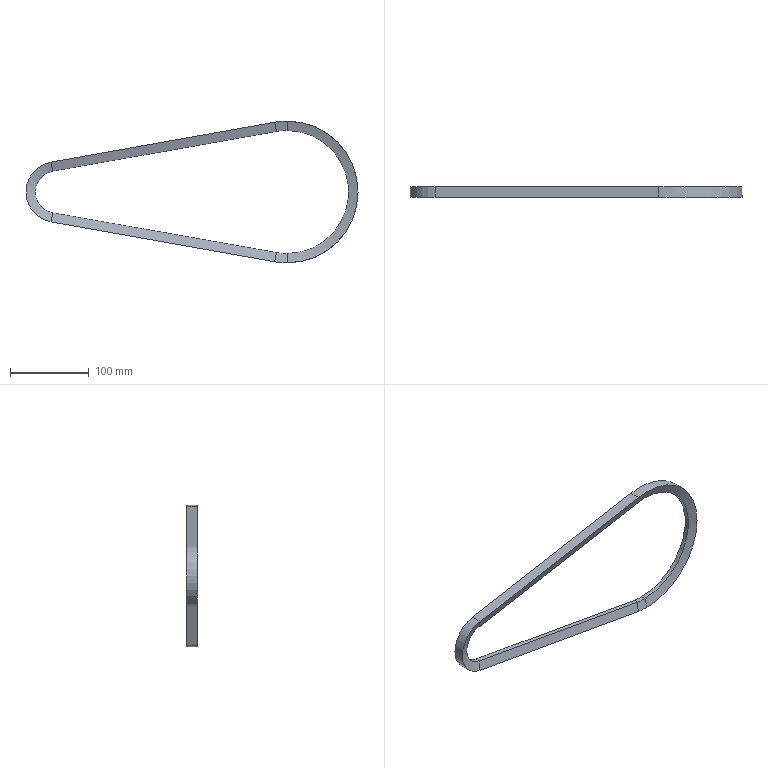Part | SolidWorks | features BaseBody 1 | 1 solid | 22 faces | box 421.873 x 13.3 x 180 mm | volume 107994 mm3 | plane 8 | cone 7 | cylinder 7 | commonest cylinder face diameters 156.432 x3 180 x2 53.781 x1 77.349 x1
STEP:
#1=CARTESIAN_POINT('',(-26.891,2.821,0.));
#2=VERTEX_POINT('',#1);
#3=CARTESIAN_POINT('',(-4.707,2.821,26.475));
#4=VERTEX_POINT('',#3);
#5=CARTESIAN_POINT('',(0.,2.821,0.));
#6=DIRECTION('',(0.,1.,0.));
#7=DIRECTION('',(0.1751,0.,-0.9846));
#8=AXIS2_PLACEMENT_3D('',#5,#6,#7);
#9=CIRCLE('',#8,26.891);
#10=EDGE_CURVE('',#2,#4,#9,.T.);
#11=ORIENTED_EDGE('',*,*,#10,.F.);
#12=CARTESIAN_POINT('',(-38.675,6.65,0.));
#13=VERTEX_POINT('',#12);
#14=CARTESIAN_POINT('',(-38.675,6.65,0.));
#15=DIRECTION('',(-0.9511,0.309,0.));
#16=VECTOR('',#15,1000.);
#17=LINE('',#14,#16);
#18=EDGE_CURVE('',#2,#13,#17,.T.);
#19=ORIENTED_EDGE('',*,*,#18,.T.);
#20=CARTESIAN_POINT('',(-6.77,6.65,38.078));
#21=VERTEX_POINT('',#20);
#22=CARTESIAN_POINT('',(0.,6.65,0.));
#23=DIRECTION('',(0.,-1.,0.));
#24=DIRECTION('',(0.1751,0.,-0.9846));
#25=AXIS2_PLACEMENT_3D('',#22,#23,#24);
#26=CIRCLE('',#25,38.675);
#27=EDGE_CURVE('',#21,#13,#26,.T.);
#28=ORIENTED_EDGE('',*,*,#27,.F.);
#29=CARTESIAN_POINT('',(-5.739,4.736,32.276));
#30=DIRECTION('',(-0.1665,0.309,0.9364));
#31=VECTOR('',#30,1000.);
#32=LINE('',#29,#31);
#33=EDGE_CURVE('',#4,#21,#32,.T.);
#34=ORIENTED_EDGE('',*,*,#33,.F.);
#35=EDGE_LOOP('',(#11,#19,#28,#34));
#36=FACE_OUTER_BOUND('',#35,.T.);
#37=CARTESIAN_POINT('',(0.,6.65,0.));
#38=DIRECTION('',(0.,1.,0.));
#39=DIRECTION('',(-1.,0.,0.));
#40=AXIS2_PLACEMENT_3D('',#37,#38,#39);
#41=CONICAL_SURFACE('',#40,38.675,1.257);
#42=ADVANCED_FACE('',(#36),#41,.F.);
#43=CARTESIAN_POINT('',(279.506,2.821,77.008));
#44=VERTEX_POINT('',#43);
#45=CARTESIAN_POINT('',(293.198,2.821,78.216));
#46=VERTEX_POINT('',#45);
#47=CARTESIAN_POINT('',(293.198,2.821,0.));
#48=DIRECTION('',(0.,1.,0.));
#49=DIRECTION('',(0.1751,0.,0.9846));
#50=AXIS2_PLACEMENT_3D('',#47,#48,#49);
#51=CIRCLE('',#50,78.216);
#52=EDGE_CURVE('',#44,#46,#51,.T.);
#53=ORIENTED_EDGE('',*,*,#52,.T.);
#54=CARTESIAN_POINT('',(293.198,-2.821,78.216));
#55=VERTEX_POINT('',#54);
#56=CARTESIAN_POINT('',(293.198,2.821,78.216));
#57=DIRECTION('',(0.,-1.,0.));
#58=VECTOR('',#57,1000.);
#59=LINE('',#56,#58);
#60=EDGE_CURVE('',#46,#55,#59,.T.);
#61=ORIENTED_EDGE('',*,*,#60,.T.);
#62=CARTESIAN_POINT('',(279.506,-2.821,77.008));
#63=VERTEX_POINT('',#62);
#64=CARTESIAN_POINT('',(293.198,-2.821,0.));
#65=DIRECTION('',(0.,1.,0.));
#66=DIRECTION('',(0.1751,0.,0.9846));
#67=AXIS2_PLACEMENT_3D('',#64,#65,#66);
#68=CIRCLE('',#67,78.216);
#69=EDGE_CURVE('',#63,#55,#68,.T.);
#70=ORIENTED_EDGE('',*,*,#69,.F.);
#71=CARTESIAN_POINT('',(279.506,0.,77.008));
#72=DIRECTION('',(0.,-1.,0.));
#73=VECTOR('',#72,1000.);
#74=LINE('',#71,#73);
#75=EDGE_CURVE('',#44,#63,#74,.T.);
#76=ORIENTED_EDGE('',*,*,#75,.F.);
#77=EDGE_LOOP('',(#53,#61,#70,#76));
#78=FACE_OUTER_BOUND('',#77,.T.);
#79=CARTESIAN_POINT('',(293.198,2.821,0.));
#80=DIRECTION('',(0.,-1.,0.));
#81=DIRECTION('',(0.,0.,-1.));
#82=AXIS2_PLACEMENT_3D('',#79,#80,#81);
#83=CYLINDRICAL_SURFACE('',#82,78.216);
#84=ADVANCED_FACE('',(#78),#83,.F.);
#85=ORIENTED_EDGE('',*,*,#60,.F.);
#86=CARTESIAN_POINT('',(293.198,2.821,-78.216));
#87=VERTEX_POINT('',#86);
#88=CARTESIAN_POINT('',(293.198,2.821,0.));
#89=DIRECTION('',(0.,1.,0.));
#90=DIRECTION('',(0.1751,0.,0.9846));
#91=AXIS2_PLACEMENT_3D('',#88,#89,#90);
#92=CIRCLE('',#91,78.216);
#93=EDGE_CURVE('',#46,#87,#92,.T.);
#94=ORIENTED_EDGE('',*,*,#93,.T.);
#95=CARTESIAN_POINT('',(293.198,-2.821,-78.216));
#96=VERTEX_POINT('',#95);
#97=CARTESIAN_POINT('',(293.198,2.821,-78.216));
#98=DIRECTION('',(0.,-1.,0.));
#99=VECTOR('',#98,1000.);
#100=LINE('',#97,#99);
#101=EDGE_CURVE('',#87,#96,#100,.T.);
#102=ORIENTED_EDGE('',*,*,#101,.T.);
#103=CARTESIAN_POINT('',(293.198,-2.821,0.));
#104=DIRECTION('',(0.,1.,0.));
#105=DIRECTION('',(0.1751,0.,0.9846));
#106=AXIS2_PLACEMENT_3D('',#103,#104,#105);
#107=CIRCLE('',#106,78.216);
#108=EDGE_CURVE('',#55,#96,#107,.T.);
#109=ORIENTED_EDGE('',*,*,#108,.F.);
#110=EDGE_LOOP('',(#85,#94,#102,#109));
#111=FACE_OUTER_BOUND('',#110,.T.);
#112=CARTESIAN_POINT('',(293.198,2.821,0.));
#113=DIRECTION('',(0.,-1.,0.));
#114=DIRECTION('',(0.,0.,-1.));
#115=AXIS2_PLACEMENT_3D('',#112,#113,#114);
#116=CYLINDRICAL_SURFACE('',#115,78.216);
#117=ADVANCED_FACE('',(#111),#116,.F.);
#118=CARTESIAN_POINT('',(277.443,6.65,-88.61));
#119=VERTEX_POINT('',#118);
#120=CARTESIAN_POINT('',(383.198,6.65,0.));
#121=VERTEX_POINT('',#120);
#122=CARTESIAN_POINT('',(293.198,6.65,0.));
#123=DIRECTION('',(0.,-1.,0.));
#124=DIRECTION('',(0.1751,0.,0.9846));
#125=AXIS2_PLACEMENT_3D('',#122,#123,#124);
#126=CIRCLE('',#125,90.);
#127=EDGE_CURVE('',#119,#121,#126,.T.);
#128=ORIENTED_EDGE('',*,*,#127,.T.);
#129=CARTESIAN_POINT('',(383.198,-6.65,0.));
#130=VERTEX_POINT('',#129);
#131=CARTESIAN_POINT('',(383.198,6.65,0.));
#132=DIRECTION('',(0.,-1.,0.));
#133=VECTOR('',#132,1000.);
#134=LINE('',#131,#133);
#135=EDGE_CURVE('',#121,#130,#134,.T.);
#136=ORIENTED_EDGE('',*,*,#135,.T.);
#137=CARTESIAN_POINT('',(293.198,-6.65,-90.));
#138=VERTEX_POINT('',#137);
#139=CARTESIAN_POINT('',(293.198,-6.65,0.));
#140=DIRECTION('',(0.,-1.,0.));
#141=DIRECTION('',(0.1751,0.,0.9846));
#142=AXIS2_PLACEMENT_3D('',#139,#140,#141);
#143=CIRCLE('',#142,90.);
#144=EDGE_CURVE('',#138,#130,#143,.T.);
#145=ORIENTED_EDGE('',*,*,#144,.F.);
#146=CARTESIAN_POINT('',(277.443,-6.65,-88.61));
#147=VERTEX_POINT('',#146);
#148=CARTESIAN_POINT('',(293.198,-6.65,0.));
#149=DIRECTION('',(0.,-1.,0.));
#150=DIRECTION('',(0.1751,0.,0.9846));
#151=AXIS2_PLACEMENT_3D('',#148,#149,#150);
#152=CIRCLE('',#151,90.);
#153=EDGE_CURVE('',#147,#138,#152,.T.);
#154=ORIENTED_EDGE('',*,*,#153,.F.);
#155=CARTESIAN_POINT('',(277.443,0.,-88.61));
#156=DIRECTION('',(0.,1.,0.));
#157=VECTOR('',#156,1000.);
#158=LINE('',#155,#157);
#159=EDGE_CURVE('',#147,#119,#158,.T.);
#160=ORIENTED_EDGE('',*,*,#159,.T.);
#161=EDGE_LOOP('',(#128,#136,#145,#154,#160));
#162=FACE_OUTER_BOUND('',#161,.T.);
#163=CARTESIAN_POINT('',(293.198,6.65,0.));
#164=DIRECTION('',(0.,-1.,0.));
#165=DIRECTION('',(1.,0.,0.));
#166=AXIS2_PLACEMENT_3D('',#163,#164,#165);
#167=CYLINDRICAL_SURFACE('',#166,90.);
#168=ADVANCED_FACE('',(#162),#167,.T.);
#169=ORIENTED_EDGE('',*,*,#69,.T.);
#170=CARTESIAN_POINT('',(293.198,-6.65,90.));
#171=VERTEX_POINT('',#170);
#172=CARTESIAN_POINT('',(293.198,-2.821,78.216));
#173=DIRECTION('',(0.,-0.309,0.9511));
#174=VECTOR('',#173,1000.);
#175=LINE('',#172,#174);
#176=EDGE_CURVE('',#55,#171,#175,.T.);
#177=ORIENTED_EDGE('',*,*,#176,.T.);
#178=CARTESIAN_POINT('',(277.443,-6.65,88.61));
#179=VERTEX_POINT('',#178);
#180=CARTESIAN_POINT('',(293.198,-6.65,0.));
#181=DIRECTION('',(0.,-1.,0.));
#182=DIRECTION('',(0.1751,0.,0.9846));
#183=AXIS2_PLACEMENT_3D('',#180,#181,#182);
#184=CIRCLE('',#183,90.);
#185=EDGE_CURVE('',#171,#179,#184,.T.);
#186=ORIENTED_EDGE('',*,*,#185,.T.);
#187=CARTESIAN_POINT('',(278.475,-4.736,82.809));
#188=DIRECTION('',(-0.1665,-0.309,0.9364));
#189=VECTOR('',#188,1000.);
#190=LINE('',#187,#189);
#191=EDGE_CURVE('',#63,#179,#190,.T.);
#192=ORIENTED_EDGE('',*,*,#191,.F.);
#193=EDGE_LOOP('',(#169,#177,#186,#192));
#194=FACE_OUTER_BOUND('',#193,.T.);
#195=CARTESIAN_POINT('',(293.198,-2.821,0.));
#196=DIRECTION('',(0.,-1.,0.));
#197=DIRECTION('',(0.,0.,-1.));
#198=AXIS2_PLACEMENT_3D('',#195,#196,#197);
#199=CONICAL_SURFACE('',#198,78.216,1.257);
#200=ADVANCED_FACE('',(#194),#199,.F.);
#201=ORIENTED_EDGE('',*,*,#176,.F.);
#202=ORIENTED_EDGE('',*,*,#108,.T.);
#203=CARTESIAN_POINT('',(293.198,-2.821,-78.216));
#204=DIRECTION('',(0.,-0.309,-0.9511));
#205=VECTOR('',#204,1000.);
#206=LINE('',#203,#205);
#207=EDGE_CURVE('',#96,#138,#206,.T.);
#208=ORIENTED_EDGE('',*,*,#207,.T.);
#209=ORIENTED_EDGE('',*,*,#144,.T.);
#210=CARTESIAN_POINT('',(293.198,-6.65,0.));
#211=DIRECTION('',(0.,-1.,0.));
#212=DIRECTION('',(0.1751,0.,0.9846));
#213=AXIS2_PLACEMENT_3D('',#210,#211,#212);
#214=CIRCLE('',#213,90.);
#215=EDGE_CURVE('',#130,#171,#214,.T.);
#216=ORIENTED_EDGE('',*,*,#215,.T.);
#217=EDGE_LOOP('',(#201,#202,#208,#209,#216));
#218=FACE_OUTER_BOUND('',#217,.T.);
#219=CARTESIAN_POINT('',(293.198,-2.821,0.));
#220=DIRECTION('',(0.,-1.,0.));
#221=DIRECTION('',(0.,0.,-1.));
#222=AXIS2_PLACEMENT_3D('',#219,#220,#221);
#223=CONICAL_SURFACE('',#222,78.216,1.257);
#224=ADVANCED_FACE('',(#218),#223,.F.);
#225=CARTESIAN_POINT('',(279.506,2.821,-77.008));
#226=VERTEX_POINT('',#225);
#227=CARTESIAN_POINT('',(278.475,4.736,-82.809));
#228=DIRECTION('',(0.1665,-0.309,0.9364));
#229=VECTOR('',#228,1000.);
#230=LINE('',#227,#229);
#231=EDGE_CURVE('',#119,#226,#230,.T.);
#232=ORIENTED_EDGE('',*,*,#231,.F.);
#233=CARTESIAN_POINT('',(-6.77,6.65,-38.078));
#234=VERTEX_POINT('',#233);
#235=CARTESIAN_POINT('',(135.337,6.65,-63.344));
#236=DIRECTION('',(0.9846,0.,-0.1751));
#237=VECTOR('',#236,1000.);
#238=LINE('',#235,#237);
#239=EDGE_CURVE('',#234,#119,#238,.T.);
#240=ORIENTED_EDGE('',*,*,#239,.F.);
#241=CARTESIAN_POINT('',(-4.707,2.821,-26.475));
#242=VERTEX_POINT('',#241);
#243=CARTESIAN_POINT('',(-5.739,4.736,-32.276));
#244=DIRECTION('',(-0.1665,0.309,-0.9364));
#245=VECTOR('',#244,1000.);
#246=LINE('',#243,#245);
#247=EDGE_CURVE('',#242,#234,#246,.T.);
#248=ORIENTED_EDGE('',*,*,#247,.F.);
#249=CARTESIAN_POINT('',(137.399,2.821,-51.742));
#250=DIRECTION('',(-0.9846,0.,0.1751));
#251=VECTOR('',#250,1000.);
#252=LINE('',#249,#251);
#253=EDGE_CURVE('',#226,#242,#252,.T.);
#254=ORIENTED_EDGE('',*,*,#253,.F.);
#255=EDGE_LOOP('',(#232,#240,#248,#254));
#256=FACE_OUTER_BOUND('',#255,.T.);
#257=CARTESIAN_POINT('',(-12.554,6.835,-37.626));
#258=DIRECTION('',(0.05409,0.9511,0.3042));
#259=DIRECTION('',(0.1665,-0.309,0.9364));
#260=AXIS2_PLACEMENT_3D('',#257,#258,#259);
#261=PLANE('',#260);
#262=ADVANCED_FACE('',(#256),#261,.T.);
#263=CARTESIAN_POINT('',(279.506,-2.821,-77.008));
#264=VERTEX_POINT('',#263);
#265=CARTESIAN_POINT('',(279.506,0.,-77.008));
#266=DIRECTION('',(0.,-1.,0.));
#267=VECTOR('',#266,1000.);
#268=LINE('',#265,#267);
#269=EDGE_CURVE('',#226,#264,#268,.T.);
#270=ORIENTED_EDGE('',*,*,#269,.F.);
#271=ORIENTED_EDGE('',*,*,#253,.T.);
#272=CARTESIAN_POINT('',(-4.707,-2.821,-26.475));
#273=VERTEX_POINT('',#272);
#274=CARTESIAN_POINT('',(-4.707,0.,-26.475));
#275=DIRECTION('',(0.,1.,0.));
#276=VECTOR('',#275,1000.);
#277=LINE('',#274,#276);
#278=EDGE_CURVE('',#273,#242,#277,.T.);
#279=ORIENTED_EDGE('',*,*,#278,.F.);
#280=CARTESIAN_POINT('',(137.399,-2.821,-51.742));
#281=DIRECTION('',(-0.9846,0.,0.1751));
#282=VECTOR('',#281,1000.);
#283=LINE('',#280,#282);
#284=EDGE_CURVE('',#264,#273,#283,.T.);
#285=ORIENTED_EDGE('',*,*,#284,.F.);
#286=EDGE_LOOP('',(#270,#271,#279,#285));
#287=FACE_OUTER_BOUND('',#286,.T.);
#288=CARTESIAN_POINT('',(-10.392,3.418,-25.465));
#289=DIRECTION('',(0.1751,0.,0.9846));
#290=DIRECTION('',(0.,-1.,0.));
#291=AXIS2_PLACEMENT_3D('',#288,#289,#290);
#292=PLANE('',#291);
#293=ADVANCED_FACE('',(#287),#292,.T.);
#294=CARTESIAN_POINT('',(277.443,6.65,88.61));
#295=VERTEX_POINT('',#294);
#296=CARTESIAN_POINT('',(278.475,4.736,82.809));
#297=DIRECTION('',(0.1665,-0.309,-0.9364));
#298=VECTOR('',#297,1000.);
#299=LINE('',#296,#298);
#300=EDGE_CURVE('',#295,#44,#299,.T.);
#301=ORIENTED_EDGE('',*,*,#300,.F.);
#302=CARTESIAN_POINT('',(293.198,6.65,0.));
#303=DIRECTION('',(0.,-1.,0.));
#304=DIRECTION('',(0.1751,0.,0.9846));
#305=AXIS2_PLACEMENT_3D('',#302,#303,#304);
#306=CIRCLE('',#305,90.);
#307=EDGE_CURVE('',#121,#295,#306,.T.);
#308=ORIENTED_EDGE('',*,*,#307,.F.);
#309=ORIENTED_EDGE('',*,*,#127,.F.);
#310=ORIENTED_EDGE('',*,*,#231,.T.);
#311=CARTESIAN_POINT('',(293.198,2.821,0.));
#312=DIRECTION('',(0.,1.,0.));
#313=DIRECTION('',(0.1751,0.,0.9846));
#314=AXIS2_PLACEMENT_3D('',#311,#312,#313);
#315=CIRCLE('',#314,78.216);
#316=EDGE_CURVE('',#87,#226,#315,.T.);
#317=ORIENTED_EDGE('',*,*,#316,.F.);
#318=ORIENTED_EDGE('',*,*,#93,.F.);
#319=ORIENTED_EDGE('',*,*,#52,.F.);
#320=EDGE_LOOP('',(#301,#308,#309,#310,#317,#318,#319));
#321=FACE_OUTER_BOUND('',#320,.T.);
#322=CARTESIAN_POINT('',(293.198,6.65,0.));
#323=DIRECTION('',(0.,1.,0.));
#324=DIRECTION('',(-1.,0.,0.));
#325=AXIS2_PLACEMENT_3D('',#322,#323,#324);
#326=CONICAL_SURFACE('',#325,90.,1.257);
#327=ADVANCED_FACE('',(#321),#326,.F.);
#328=ORIENTED_EDGE('',*,*,#159,.F.);
#329=CARTESIAN_POINT('',(-6.77,-6.65,-38.078));
#330=VERTEX_POINT('',#329);
#331=CARTESIAN_POINT('',(135.337,-6.65,-63.344));
#332=DIRECTION('',(0.9846,0.,-0.1751));
#333=VECTOR('',#332,1000.);
#334=LINE('',#331,#333);
#335=EDGE_CURVE('',#330,#147,#334,.T.);
#336=ORIENTED_EDGE('',*,*,#335,.F.);
#337=CARTESIAN_POINT('',(-6.77,0.,-38.078));
#338=DIRECTION('',(0.,-1.,0.));
#339=VECTOR('',#338,1000.);
#340=LINE('',#337,#339);
#341=EDGE_CURVE('',#234,#330,#340,.T.);
#342=ORIENTED_EDGE('',*,*,#341,.F.);
#343=ORIENTED_EDGE('',*,*,#239,.T.);
#344=EDGE_LOOP('',(#328,#336,#342,#343));
#345=FACE_OUTER_BOUND('',#344,.T.);
#346=CARTESIAN_POINT('',(-12.454,-7.247,-37.067));
#347=DIRECTION('',(-0.1751,0.,-0.9846));
#348=DIRECTION('',(0.,1.,0.));
#349=AXIS2_PLACEMENT_3D('',#346,#347,#348);
#350=PLANE('',#349);
#351=ADVANCED_FACE('',(#345),#350,.T.);
#352=ORIENTED_EDGE('',*,*,#18,.F.);
#353=CARTESIAN_POINT('',(0.,2.821,0.));
#354=DIRECTION('',(0.,1.,0.));
#355=DIRECTION('',(0.1751,0.,-0.9846));
#356=AXIS2_PLACEMENT_3D('',#353,#354,#355);
#357=CIRCLE('',#356,26.891);
#358=EDGE_CURVE('',#242,#2,#357,.T.);
#359=ORIENTED_EDGE('',*,*,#358,.F.);
#360=ORIENTED_EDGE('',*,*,#247,.T.);
#361=CARTESIAN_POINT('',(0.,6.65,0.));
#362=DIRECTION('',(0.,-1.,0.));
#363=DIRECTION('',(0.1751,0.,-0.9846));
#364=AXIS2_PLACEMENT_3D('',#361,#362,#363);
#365=CIRCLE('',#364,38.675);
#366=EDGE_CURVE('',#13,#234,#365,.T.);
#367=ORIENTED_EDGE('',*,*,#366,.F.);
#368=EDGE_LOOP('',(#352,#359,#360,#367));
#369=FACE_OUTER_BOUND('',#368,.T.);
#370=CARTESIAN_POINT('',(0.,6.65,0.));
#371=DIRECTION('',(0.,1.,0.));
#372=DIRECTION('',(-1.,0.,0.));
#373=AXIS2_PLACEMENT_3D('',#370,#371,#372);
#374=CONICAL_SURFACE('',#373,38.675,1.257);
#375=ADVANCED_FACE('',(#369),#374,.F.);
#376=CARTESIAN_POINT('',(278.475,-4.736,-82.809));
#377=DIRECTION('',(-0.1665,-0.309,-0.9364));
#378=VECTOR('',#377,1000.);
#379=LINE('',#376,#378);
#380=EDGE_CURVE('',#264,#147,#379,.T.);
#381=ORIENTED_EDGE('',*,*,#380,.F.);
#382=ORIENTED_EDGE('',*,*,#284,.T.);
#383=CARTESIAN_POINT('',(-5.739,-4.736,-32.276));
#384=DIRECTION('',(0.1665,0.309,0.9364));
#385=VECTOR('',#384,1000.);
#386=LINE('',#383,#385);
#387=EDGE_CURVE('',#330,#273,#386,.T.);
#388=ORIENTED_EDGE('',*,*,#387,.F.);
#389=ORIENTED_EDGE('',*,*,#335,.T.);
#390=EDGE_LOOP('',(#381,#382,#388,#389));
#391=FACE_OUTER_BOUND('',#390,.T.);
#392=CARTESIAN_POINT('',(-10.292,-2.637,-24.905));
#393=DIRECTION('',(0.05409,-0.9511,0.3042));
#394=DIRECTION('',(-0.1665,-0.309,-0.9364));
#395=AXIS2_PLACEMENT_3D('',#392,#393,#394);
#396=PLANE('',#395);
#397=ADVANCED_FACE('',(#391),#396,.T.);
#398=ORIENTED_EDGE('',*,*,#101,.F.);
#399=ORIENTED_EDGE('',*,*,#316,.T.);
#400=ORIENTED_EDGE('',*,*,#269,.T.);
#401=CARTESIAN_POINT('',(293.198,-2.821,0.));
#402=DIRECTION('',(0.,1.,0.));
#403=DIRECTION('',(0.1751,0.,0.9846));
#404=AXIS2_PLACEMENT_3D('',#401,#402,#403);
#405=CIRCLE('',#404,78.216);
#406=EDGE_CURVE('',#96,#264,#405,.T.);
#407=ORIENTED_EDGE('',*,*,#406,.F.);
#408=EDGE_LOOP('',(#398,#399,#400,#407));
#409=FACE_OUTER_BOUND('',#408,.T.);
#410=CARTESIAN_POINT('',(293.198,2.821,0.));
#411=DIRECTION('',(0.,-1.,0.));
#412=DIRECTION('',(0.,0.,-1.));
#413=AXIS2_PLACEMENT_3D('',#410,#411,#412);
#414=CYLINDRICAL_SURFACE('',#413,78.216);
#415=ADVANCED_FACE('',(#409),#414,.F.);
#416=ORIENTED_EDGE('',*,*,#278,.T.);
#417=ORIENTED_EDGE('',*,*,#358,.T.);
#418=ORIENTED_EDGE('',*,*,#10,.T.);
#419=CARTESIAN_POINT('',(-4.707,-2.821,26.475));
#420=VERTEX_POINT('',#419);
#421=CARTESIAN_POINT('',(-4.707,0.,26.475));
#422=DIRECTION('',(0.,1.,0.));
#423=VECTOR('',#422,1000.);
#424=LINE('',#421,#423);
#425=EDGE_CURVE('',#420,#4,#424,.T.);
#426=ORIENTED_EDGE('',*,*,#425,.F.);
#427=CARTESIAN_POINT('',(0.,-2.821,0.));
#428=DIRECTION('',(0.,1.,0.));
#429=DIRECTION('',(0.1751,0.,-0.9846));
#430=AXIS2_PLACEMENT_3D('',#427,#428,#429);
#431=CIRCLE('',#430,26.891);
#432=EDGE_CURVE('',#273,#420,#431,.T.);
#433=ORIENTED_EDGE('',*,*,#432,.F.);
#434=EDGE_LOOP('',(#416,#417,#418,#426,#433));
#435=FACE_OUTER_BOUND('',#434,.T.);
#436=CARTESIAN_POINT('',(0.,2.821,0.));
#437=DIRECTION('',(0.,-1.,0.));
#438=DIRECTION('',(0.,0.,-1.));
#439=AXIS2_PLACEMENT_3D('',#436,#437,#438);
#440=CYLINDRICAL_SURFACE('',#439,26.891);
#441=ADVANCED_FACE('',(#435),#440,.F.);
#442=ORIENTED_EDGE('',*,*,#33,.T.);
#443=CARTESIAN_POINT('',(135.337,6.65,63.344));
#444=DIRECTION('',(-0.9846,0.,-0.1751));
#445=VECTOR('',#444,1000.);
#446=LINE('',#443,#445);
#447=EDGE_CURVE('',#295,#21,#446,.T.);
#448=ORIENTED_EDGE('',*,*,#447,.F.);
#449=ORIENTED_EDGE('',*,*,#300,.T.);
#450=CARTESIAN_POINT('',(137.399,2.821,51.742));
#451=DIRECTION('',(0.9846,0.,0.1751));
#452=VECTOR('',#451,1000.);
#453=LINE('',#450,#452);
#454=EDGE_CURVE('',#4,#44,#453,.T.);
#455=ORIENTED_EDGE('',*,*,#454,.F.);
#456=EDGE_LOOP('',(#442,#448,#449,#455));
#457=FACE_OUTER_BOUND('',#456,.T.);
#458=CARTESIAN_POINT('',(283.028,6.835,90.18));
#459=DIRECTION('',(0.05409,0.9511,-0.3042));
#460=DIRECTION('',(0.1665,-0.309,-0.9364));
#461=AXIS2_PLACEMENT_3D('',#458,#459,#460);
#462=PLANE('',#461);
#463=ADVANCED_FACE('',(#457),#462,.T.);
#464=ORIENTED_EDGE('',*,*,#135,.F.);
#465=ORIENTED_EDGE('',*,*,#307,.T.);
#466=CARTESIAN_POINT('',(277.443,0.,88.61));
#467=DIRECTION('',(0.,1.,0.));
#468=VECTOR('',#467,1000.);
#469=LINE('',#466,#468);
#470=EDGE_CURVE('',#179,#295,#469,.T.);
#471=ORIENTED_EDGE('',*,*,#470,.F.);
#472=ORIENTED_EDGE('',*,*,#185,.F.);
#473=ORIENTED_EDGE('',*,*,#215,.F.);
#474=EDGE_LOOP('',(#464,#465,#471,#472,#473));
#475=FACE_OUTER_BOUND('',#474,.T.);
#476=CARTESIAN_POINT('',(293.198,6.65,0.));
#477=DIRECTION('',(0.,-1.,0.));
#478=DIRECTION('',(1.,0.,0.));
#479=AXIS2_PLACEMENT_3D('',#476,#477,#478);
#480=CYLINDRICAL_SURFACE('',#479,90.);
#481=ADVANCED_FACE('',(#475),#480,.T.);
#482=ORIENTED_EDGE('',*,*,#341,.T.);
#483=CARTESIAN_POINT('',(-6.77,-6.65,38.078));
#484=VERTEX_POINT('',#483);
#485=CARTESIAN_POINT('',(0.,-6.65,0.));
#486=DIRECTION('',(0.,-1.,0.));
#487=DIRECTION('',(0.1751,0.,-0.9846));
#488=AXIS2_PLACEMENT_3D('',#485,#486,#487);
#489=CIRCLE('',#488,38.675);
#490=EDGE_CURVE('',#484,#330,#489,.T.);
#491=ORIENTED_EDGE('',*,*,#490,.F.);
#492=CARTESIAN_POINT('',(-6.77,0.,38.078));
#493=DIRECTION('',(0.,-1.,0.));
#494=VECTOR('',#493,1000.);
#495=LINE('',#492,#494);
#496=EDGE_CURVE('',#21,#484,#495,.T.);
#497=ORIENTED_EDGE('',*,*,#496,.F.);
#498=ORIENTED_EDGE('',*,*,#27,.T.);
#499=ORIENTED_EDGE('',*,*,#366,.T.);
#500=EDGE_LOOP('',(#482,#491,#497,#498,#499));
#501=FACE_OUTER_BOUND('',#500,.T.);
#502=CARTESIAN_POINT('',(0.,6.65,0.));
#503=DIRECTION('',(0.,-1.,0.));
#504=DIRECTION('',(0.,0.,-1.));
#505=AXIS2_PLACEMENT_3D('',#502,#503,#504);
#506=CYLINDRICAL_SURFACE('',#505,38.675);
#507=ADVANCED_FACE('',(#501),#506,.T.);
#508=ORIENTED_EDGE('',*,*,#207,.F.);
#509=ORIENTED_EDGE('',*,*,#406,.T.);
#510=ORIENTED_EDGE('',*,*,#380,.T.);
#511=ORIENTED_EDGE('',*,*,#153,.T.);
#512=EDGE_LOOP('',(#508,#509,#510,#511));
#513=FACE_OUTER_BOUND('',#512,.T.);
#514=CARTESIAN_POINT('',(293.198,-2.821,0.));
#515=DIRECTION('',(0.,-1.,0.));
#516=DIRECTION('',(0.,0.,-1.));
#517=AXIS2_PLACEMENT_3D('',#514,#515,#516);
#518=CONICAL_SURFACE('',#517,78.216,1.257);
#519=ADVANCED_FACE('',(#513),#518,.F.);
#520=ORIENTED_EDGE('',*,*,#387,.T.);
#521=ORIENTED_EDGE('',*,*,#432,.T.);
#522=CARTESIAN_POINT('',(-5.739,-4.736,32.276));
#523=DIRECTION('',(0.1665,0.309,-0.9364));
#524=VECTOR('',#523,1000.);
#525=LINE('',#522,#524);
#526=EDGE_CURVE('',#484,#420,#525,.T.);
#527=ORIENTED_EDGE('',*,*,#526,.F.);
#528=ORIENTED_EDGE('',*,*,#490,.T.);
#529=EDGE_LOOP('',(#520,#521,#527,#528));
#530=FACE_OUTER_BOUND('',#529,.T.);
#531=CARTESIAN_POINT('',(0.,-2.821,0.));
#532=DIRECTION('',(0.,-1.,0.));
#533=DIRECTION('',(0.,0.,-1.));
#534=AXIS2_PLACEMENT_3D('',#531,#532,#533);
#535=CONICAL_SURFACE('',#534,26.891,1.257);
#536=ADVANCED_FACE('',(#530),#535,.F.);
#537=ORIENTED_EDGE('',*,*,#425,.T.);
#538=ORIENTED_EDGE('',*,*,#454,.T.);
#539=ORIENTED_EDGE('',*,*,#75,.T.);
#540=CARTESIAN_POINT('',(137.399,-2.821,51.742));
#541=DIRECTION('',(0.9846,0.,0.1751));
#542=VECTOR('',#541,1000.);
#543=LINE('',#540,#542);
#544=EDGE_CURVE('',#420,#63,#543,.T.);
#545=ORIENTED_EDGE('',*,*,#544,.F.);
#546=EDGE_LOOP('',(#537,#538,#539,#545));
#547=FACE_OUTER_BOUND('',#546,.T.);
#548=CARTESIAN_POINT('',(285.19,3.418,78.019));
#549=DIRECTION('',(0.1751,0.,-0.9846));
#550=DIRECTION('',(0.,-1.,0.));
#551=AXIS2_PLACEMENT_3D('',#548,#549,#550);
#552=PLANE('',#551);
#553=ADVANCED_FACE('',(#547),#552,.T.);
#554=ORIENTED_EDGE('',*,*,#496,.T.);
#555=CARTESIAN_POINT('',(135.337,-6.65,63.344));
#556=DIRECTION('',(-0.9846,0.,-0.1751));
#557=VECTOR('',#556,1000.);
#558=LINE('',#555,#557);
#559=EDGE_CURVE('',#179,#484,#558,.T.);
#560=ORIENTED_EDGE('',*,*,#559,.F.);
#561=ORIENTED_EDGE('',*,*,#470,.T.);
#562=ORIENTED_EDGE('',*,*,#447,.T.);
#563=EDGE_LOOP('',(#554,#560,#561,#562));
#564=FACE_OUTER_BOUND('',#563,.T.);
#565=CARTESIAN_POINT('',(283.127,-7.247,89.621));
#566=DIRECTION('',(-0.1751,0.,0.9846));
#567=DIRECTION('',(0.,1.,0.));
#568=AXIS2_PLACEMENT_3D('',#565,#566,#567);
#569=PLANE('',#568);
#570=ADVANCED_FACE('',(#564),#569,.T.);
#571=ORIENTED_EDGE('',*,*,#526,.T.);
#572=ORIENTED_EDGE('',*,*,#544,.T.);
#573=ORIENTED_EDGE('',*,*,#191,.T.);
#574=ORIENTED_EDGE('',*,*,#559,.T.);
#575=EDGE_LOOP('',(#571,#572,#573,#574));
#576=FACE_OUTER_BOUND('',#575,.T.);
#577=CARTESIAN_POINT('',(285.29,-2.637,77.459));
#578=DIRECTION('',(0.05409,-0.9511,-0.3042));
#579=DIRECTION('',(-0.1665,-0.309,0.9364));
#580=AXIS2_PLACEMENT_3D('',#577,#578,#579);
#581=PLANE('',#580);
#582=ADVANCED_FACE('',(#576),#581,.T.);
#583=CLOSED_SHELL('',(#42,#84,#117,#168,#200,#224,#262,#293,#327,#351,#375,#397,#415,#441,#463,#481,#507,#519,#536,#553,#570,#582));
#584=MANIFOLD_SOLID_BREP('',#583);
#585=CARTESIAN_POINT('',(0.,0.,0.));
#586=DIRECTION('',(0.,0.,1.));
#587=DIRECTION('',(1.,0.,0.));
#588=AXIS2_PLACEMENT_3D('',#585,#586,#587);
#589=(LENGTH_UNIT()NAMED_UNIT(*)SI_UNIT(.MILLI.,.METRE.));
#590=UNCERTAINTY_MEASURE_WITH_UNIT(LENGTH_MEASURE(0.00001),#589,'','');
#591=(NAMED_UNIT(*)PLANE_ANGLE_UNIT()SI_UNIT($,.RADIAN.));
#592=(NAMED_UNIT(*)SI_UNIT($,.STERADIAN.)SOLID_ANGLE_UNIT());
#593=(GEOMETRIC_REPRESENTATION_CONTEXT(3)GLOBAL_UNCERTAINTY_ASSIGNED_CONTEXT((#590))GLOBAL_UNIT_ASSIGNED_CONTEXT((#589,#591,#592))REPRESENTATION_CONTEXT('',''));
#594=ADVANCED_BREP_SHAPE_REPRESENTATION('',(#584,#588),#593);